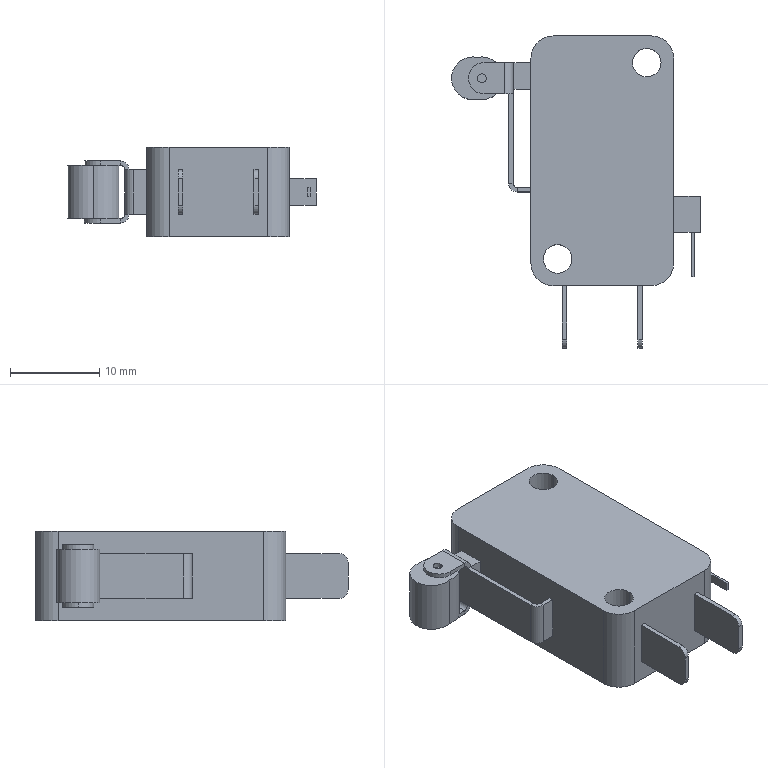Part | SolidWorks | features ICE 3, BaseBody 1 | 1 solid | 85 faces | box 27.9 x 35 x 10 mm | volume 4554 mm3 | plane 58 | cylinder 27 | commonest cylinder face diameters 1 x7 2 x7 3.2 x4 5 x4 3.5 x3 4.8 x2